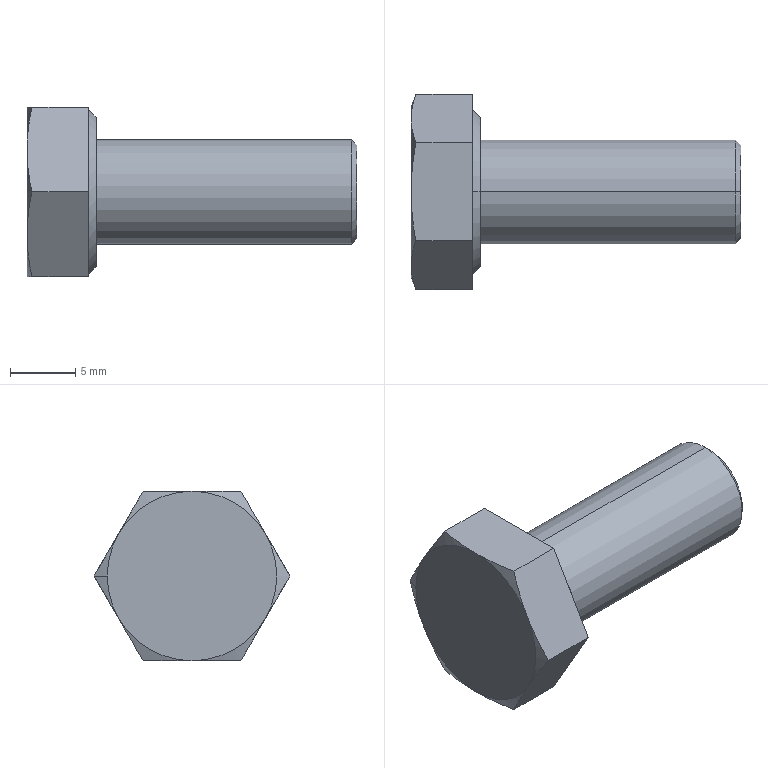Part | SolidWorks | features BaseBody 1, MoveFace 1 | 1 solid | 23 faces | box 25.3 x 15.011 x 13 mm | volume 1758 mm3 | cone 11 | plane 10 | cylinder 2 | commonest cylinder face diameters 8 x2
STEP:
#1=CARTESIAN_POINT('',(24.9,0.,4.));
#2=VERTEX_POINT('',#1);
#3=CARTESIAN_POINT('',(24.9,0.,-4.));
#4=VERTEX_POINT('',#3);
#5=CARTESIAN_POINT('',(24.9,0.,0.));
#6=DIRECTION('',(-1.,0.,0.));
#7=DIRECTION('',(0.,0.,1.));
#8=AXIS2_PLACEMENT_3D('',#5,#6,#7);
#9=CIRCLE('',#8,4.);
#10=EDGE_CURVE('',#2,#4,#9,.T.);
#11=ORIENTED_EDGE('',*,*,#10,.T.);
#12=CARTESIAN_POINT('',(5.3,0.,-4.));
#13=VERTEX_POINT('',#12);
#14=CARTESIAN_POINT('',(45.3,0.,-4.));
#15=DIRECTION('',(-1.,0.,0.));
#16=VECTOR('',#15,1000.);
#17=LINE('',#14,#16);
#18=EDGE_CURVE('',#4,#13,#17,.T.);
#19=ORIENTED_EDGE('',*,*,#18,.T.);
#20=CARTESIAN_POINT('',(5.3,0.,4.));
#21=VERTEX_POINT('',#20);
#22=CARTESIAN_POINT('',(5.3,0.,0.));
#23=DIRECTION('',(1.,0.,0.));
#24=DIRECTION('',(0.,0.,1.));
#25=AXIS2_PLACEMENT_3D('',#22,#23,#24);
#26=CIRCLE('',#25,4.);
#27=EDGE_CURVE('',#13,#21,#26,.T.);
#28=ORIENTED_EDGE('',*,*,#27,.T.);
#29=CARTESIAN_POINT('',(45.3,0.,4.));
#30=DIRECTION('',(-1.,0.,0.));
#31=VECTOR('',#30,1000.);
#32=LINE('',#29,#31);
#33=EDGE_CURVE('',#2,#21,#32,.T.);
#34=ORIENTED_EDGE('',*,*,#33,.F.);
#35=EDGE_LOOP('',(#11,#19,#28,#34));
#36=FACE_OUTER_BOUND('',#35,.T.);
#37=CARTESIAN_POINT('',(45.3,0.,0.));
#38=DIRECTION('',(-1.,0.,0.));
#39=DIRECTION('',(0.,0.,1.));
#40=AXIS2_PLACEMENT_3D('',#37,#38,#39);
#41=CYLINDRICAL_SURFACE('',#40,4.);
#42=ADVANCED_FACE('',(#36),#41,.T.);
#43=CARTESIAN_POINT('',(25.3,0.,3.6));
#44=VERTEX_POINT('',#43);
#45=CARTESIAN_POINT('',(25.3,0.,-3.6));
#46=VERTEX_POINT('',#45);
#47=CARTESIAN_POINT('',(25.3,0.,0.));
#48=DIRECTION('',(-1.,0.,0.));
#49=DIRECTION('',(0.,0.,1.));
#50=AXIS2_PLACEMENT_3D('',#47,#48,#49);
#51=CIRCLE('',#50,3.6);
#52=EDGE_CURVE('',#44,#46,#51,.T.);
#53=ORIENTED_EDGE('',*,*,#52,.T.);
#54=CARTESIAN_POINT('',(24.9,0.,-4.));
#55=DIRECTION('',(-0.7071,0.,-0.7071));
#56=VECTOR('',#55,1000.);
#57=LINE('',#54,#56);
#58=EDGE_CURVE('',#46,#4,#57,.T.);
#59=ORIENTED_EDGE('',*,*,#58,.T.);
#60=ORIENTED_EDGE('',*,*,#10,.F.);
#61=CARTESIAN_POINT('',(24.9,0.,4.));
#62=DIRECTION('',(-0.7071,0.,0.7071));
#63=VECTOR('',#62,1000.);
#64=LINE('',#61,#63);
#65=EDGE_CURVE('',#44,#2,#64,.T.);
#66=ORIENTED_EDGE('',*,*,#65,.F.);
#67=EDGE_LOOP('',(#53,#59,#60,#66));
#68=FACE_OUTER_BOUND('',#67,.T.);
#69=CARTESIAN_POINT('',(24.9,0.,0.));
#70=DIRECTION('',(-1.,0.,0.));
#71=DIRECTION('',(0.,0.,1.));
#72=AXIS2_PLACEMENT_3D('',#69,#70,#71);
#73=CONICAL_SURFACE('',#72,4.,0.7854);
#74=ADVANCED_FACE('',(#68),#73,.T.);
#75=CARTESIAN_POINT('',(5.3,0.,5.735));
#76=VERTEX_POINT('',#75);
#77=CARTESIAN_POINT('',(5.3,0.,-5.735));
#78=VERTEX_POINT('',#77);
#79=CARTESIAN_POINT('',(5.3,0.,0.));
#80=DIRECTION('',(-1.,0.,0.));
#81=DIRECTION('',(0.,0.,1.));
#82=AXIS2_PLACEMENT_3D('',#79,#80,#81);
#83=CIRCLE('',#82,5.735);
#84=EDGE_CURVE('',#76,#78,#83,.T.);
#85=ORIENTED_EDGE('',*,*,#84,.T.);
#86=CARTESIAN_POINT('',(4.7,0.,-6.335));
#87=VERTEX_POINT('',#86);
#88=CARTESIAN_POINT('',(4.7,0.,-6.335));
#89=DIRECTION('',(-0.7071,0.,-0.7071));
#90=VECTOR('',#89,1000.);
#91=LINE('',#88,#90);
#92=EDGE_CURVE('',#78,#87,#91,.T.);
#93=ORIENTED_EDGE('',*,*,#92,.T.);
#94=CARTESIAN_POINT('',(4.7,0.,6.335));
#95=VERTEX_POINT('',#94);
#96=CARTESIAN_POINT('',(4.7,0.,0.));
#97=DIRECTION('',(1.,0.,0.));
#98=DIRECTION('',(0.,0.,1.));
#99=AXIS2_PLACEMENT_3D('',#96,#97,#98);
#100=CIRCLE('',#99,6.335);
#101=EDGE_CURVE('',#87,#95,#100,.T.);
#102=ORIENTED_EDGE('',*,*,#101,.T.);
#103=CARTESIAN_POINT('',(4.7,0.,6.335));
#104=DIRECTION('',(-0.7071,0.,0.7071));
#105=VECTOR('',#104,1000.);
#106=LINE('',#103,#105);
#107=EDGE_CURVE('',#76,#95,#106,.T.);
#108=ORIENTED_EDGE('',*,*,#107,.F.);
#109=EDGE_LOOP('',(#85,#93,#102,#108));
#110=FACE_OUTER_BOUND('',#109,.T.);
#111=CARTESIAN_POINT('',(4.7,0.,0.));
#112=DIRECTION('',(-1.,0.,0.));
#113=DIRECTION('',(0.,0.,1.));
#114=AXIS2_PLACEMENT_3D('',#111,#112,#113);
#115=CONICAL_SURFACE('',#114,6.335,0.7854);
#116=ADVANCED_FACE('',(#110),#115,.T.);
#117=CARTESIAN_POINT('',(0.,5.629,-3.25));
#118=VERTEX_POINT('',#117);
#119=CARTESIAN_POINT('',(0.,6.5,0.));
#120=VERTEX_POINT('',#119);
#121=CARTESIAN_POINT('',(0.,0.,0.));
#122=DIRECTION('',(1.,0.,0.));
#123=DIRECTION('',(0.,1.,0.));
#124=AXIS2_PLACEMENT_3D('',#121,#122,#123);
#125=CIRCLE('',#124,6.5);
#126=EDGE_CURVE('',#118,#120,#125,.T.);
#127=ORIENTED_EDGE('',*,*,#126,.T.);
#128=CARTESIAN_POINT('',(0.366,7.506,0.));
#129=VERTEX_POINT('',#128);
#130=CARTESIAN_POINT('',(0.3682,7.512,0.));
#131=DIRECTION('',(0.342,0.9397,0.));
#132=VECTOR('',#131,1000.);
#133=LINE('',#130,#132);
#134=EDGE_CURVE('',#120,#129,#133,.T.);
#135=ORIENTED_EDGE('',*,*,#134,.T.);
#136=CARTESIAN_POINT('',(0.366,7.506,0.));
#137=CARTESIAN_POINT('',(0.1402,6.885,-1.075));
#138=CARTESIAN_POINT('',(0.,6.261,-2.156));
#139=CARTESIAN_POINT('',(0.,5.629,-3.25));
#140=B_SPLINE_CURVE_WITH_KNOTS('',3,(#136,#137,#138,#139),.UNSPECIFIED.,.F.,.F.,(4,4),(0.,0.003771),.UNSPECIFIED.);
#141=EDGE_CURVE('',#129,#118,#140,.T.);
#142=ORIENTED_EDGE('',*,*,#141,.T.);
#143=EDGE_LOOP('',(#127,#135,#142));
#144=FACE_OUTER_BOUND('',#143,.T.);
#145=CARTESIAN_POINT('',(0.3682,0.,0.));
#146=DIRECTION('',(1.,0.,0.));
#147=DIRECTION('',(0.,1.,0.));
#148=AXIS2_PLACEMENT_3D('',#145,#146,#147);
#149=CONICAL_SURFACE('',#148,7.512,1.222);
#150=ADVANCED_FACE('',(#144),#149,.T.);
#151=ORIENTED_EDGE('',*,*,#18,.F.);
#152=CARTESIAN_POINT('',(24.9,0.,0.));
#153=DIRECTION('',(-1.,0.,0.));
#154=DIRECTION('',(0.,0.,1.));
#155=AXIS2_PLACEMENT_3D('',#152,#153,#154);
#156=CIRCLE('',#155,4.);
#157=EDGE_CURVE('',#4,#2,#156,.T.);
#158=ORIENTED_EDGE('',*,*,#157,.T.);
#159=ORIENTED_EDGE('',*,*,#33,.T.);
#160=CARTESIAN_POINT('',(5.3,0.,0.));
#161=DIRECTION('',(1.,0.,0.));
#162=DIRECTION('',(0.,0.,1.));
#163=AXIS2_PLACEMENT_3D('',#160,#161,#162);
#164=CIRCLE('',#163,4.);
#165=EDGE_CURVE('',#21,#13,#164,.T.);
#166=ORIENTED_EDGE('',*,*,#165,.T.);
#167=EDGE_LOOP('',(#151,#158,#159,#166));
#168=FACE_OUTER_BOUND('',#167,.T.);
#169=CARTESIAN_POINT('',(45.3,0.,0.));
#170=DIRECTION('',(-1.,0.,0.));
#171=DIRECTION('',(0.,0.,1.));
#172=AXIS2_PLACEMENT_3D('',#169,#170,#171);
#173=CYLINDRICAL_SURFACE('',#172,4.);
#174=ADVANCED_FACE('',(#168),#173,.T.);
#175=ORIENTED_EDGE('',*,*,#165,.F.);
#176=ORIENTED_EDGE('',*,*,#27,.F.);
#177=EDGE_LOOP('',(#175,#176));
#178=FACE_BOUND('',#177,.T.);
#179=ORIENTED_EDGE('',*,*,#84,.F.);
#180=CARTESIAN_POINT('',(5.3,0.,0.));
#181=DIRECTION('',(-1.,0.,0.));
#182=DIRECTION('',(0.,0.,1.));
#183=AXIS2_PLACEMENT_3D('',#180,#181,#182);
#184=CIRCLE('',#183,5.735);
#185=EDGE_CURVE('',#78,#76,#184,.T.);
#186=ORIENTED_EDGE('',*,*,#185,.F.);
#187=EDGE_LOOP('',(#179,#186));
#188=FACE_OUTER_BOUND('',#187,.T.);
#189=CARTESIAN_POINT('',(5.3,0.,13.));
#190=DIRECTION('',(-1.,0.,0.));
#191=DIRECTION('',(0.,0.,1.));
#192=AXIS2_PLACEMENT_3D('',#189,#190,#191);
#193=PLANE('',#192);
#194=ADVANCED_FACE('',(#178,#188),#193,.F.);
#195=ORIENTED_EDGE('',*,*,#58,.F.);
#196=CARTESIAN_POINT('',(25.3,0.,0.));
#197=DIRECTION('',(-1.,0.,0.));
#198=DIRECTION('',(0.,0.,1.));
#199=AXIS2_PLACEMENT_3D('',#196,#197,#198);
#200=CIRCLE('',#199,3.6);
#201=EDGE_CURVE('',#46,#44,#200,.T.);
#202=ORIENTED_EDGE('',*,*,#201,.T.);
#203=ORIENTED_EDGE('',*,*,#65,.T.);
#204=ORIENTED_EDGE('',*,*,#157,.F.);
#205=EDGE_LOOP('',(#195,#202,#203,#204));
#206=FACE_OUTER_BOUND('',#205,.T.);
#207=CARTESIAN_POINT('',(24.9,0.,0.));
#208=DIRECTION('',(-1.,0.,0.));
#209=DIRECTION('',(0.,0.,1.));
#210=AXIS2_PLACEMENT_3D('',#207,#208,#209);
#211=CONICAL_SURFACE('',#210,4.,0.7854);
#212=ADVANCED_FACE('',(#206),#211,.T.);
#213=ORIENTED_EDGE('',*,*,#92,.F.);
#214=ORIENTED_EDGE('',*,*,#185,.T.);
#215=ORIENTED_EDGE('',*,*,#107,.T.);
#216=CARTESIAN_POINT('',(4.7,0.,0.));
#217=DIRECTION('',(1.,0.,0.));
#218=DIRECTION('',(0.,0.,1.));
#219=AXIS2_PLACEMENT_3D('',#216,#217,#218);
#220=CIRCLE('',#219,6.335);
#221=EDGE_CURVE('',#95,#87,#220,.T.);
#222=ORIENTED_EDGE('',*,*,#221,.T.);
#223=EDGE_LOOP('',(#213,#214,#215,#222));
#224=FACE_OUTER_BOUND('',#223,.T.);
#225=CARTESIAN_POINT('',(4.7,0.,0.));
#226=DIRECTION('',(-1.,0.,0.));
#227=DIRECTION('',(0.,0.,1.));
#228=AXIS2_PLACEMENT_3D('',#225,#226,#227);
#229=CONICAL_SURFACE('',#228,6.335,0.7854);
#230=ADVANCED_FACE('',(#224),#229,.T.);
#231=ORIENTED_EDGE('',*,*,#52,.F.);
#232=ORIENTED_EDGE('',*,*,#201,.F.);
#233=EDGE_LOOP('',(#231,#232));
#234=FACE_OUTER_BOUND('',#233,.T.);
#235=CARTESIAN_POINT('',(25.3,0.,0.));
#236=DIRECTION('',(1.,0.,0.));
#237=DIRECTION('',(0.,0.,-1.));
#238=AXIS2_PLACEMENT_3D('',#235,#236,#237);
#239=PLANE('',#238);
#240=ADVANCED_FACE('',(#234),#239,.T.);
#241=CARTESIAN_POINT('',(4.7,7.506,0.));
#242=VERTEX_POINT('',#241);
#243=CARTESIAN_POINT('',(4.7,3.753,6.5));
#244=VERTEX_POINT('',#243);
#245=CARTESIAN_POINT('',(4.7,7.506,0.));
#246=DIRECTION('',(0.,-0.5,0.866));
#247=VECTOR('',#246,1000.);
#248=LINE('',#245,#247);
#249=EDGE_CURVE('',#242,#244,#248,.T.);
#250=ORIENTED_EDGE('',*,*,#249,.T.);
#251=CARTESIAN_POINT('',(4.7,-3.753,6.5));
#252=VERTEX_POINT('',#251);
#253=CARTESIAN_POINT('',(4.7,6.335,6.5));
#254=DIRECTION('',(0.,-1.,0.));
#255=VECTOR('',#254,1000.);
#256=LINE('',#253,#255);
#257=EDGE_CURVE('',#244,#252,#256,.T.);
#258=ORIENTED_EDGE('',*,*,#257,.T.);
#259=CARTESIAN_POINT('',(4.7,-7.506,0.));
#260=VERTEX_POINT('',#259);
#261=CARTESIAN_POINT('',(4.7,-3.753,6.5));
#262=DIRECTION('',(0.,-0.5,-0.866));
#263=VECTOR('',#262,1000.);
#264=LINE('',#261,#263);
#265=EDGE_CURVE('',#252,#260,#264,.T.);
#266=ORIENTED_EDGE('',*,*,#265,.T.);
#267=CARTESIAN_POINT('',(4.7,-3.753,-6.5));
#268=VERTEX_POINT('',#267);
#269=CARTESIAN_POINT('',(4.7,-7.506,0.));
#270=DIRECTION('',(0.,0.5,-0.866));
#271=VECTOR('',#270,1000.);
#272=LINE('',#269,#271);
#273=EDGE_CURVE('',#260,#268,#272,.T.);
#274=ORIENTED_EDGE('',*,*,#273,.T.);
#275=CARTESIAN_POINT('',(4.7,3.753,-6.5));
#276=VERTEX_POINT('',#275);
#277=CARTESIAN_POINT('',(4.7,6.335,-6.5));
#278=DIRECTION('',(0.,1.,0.));
#279=VECTOR('',#278,1000.);
#280=LINE('',#277,#279);
#281=EDGE_CURVE('',#268,#276,#280,.T.);
#282=ORIENTED_EDGE('',*,*,#281,.T.);
#283=CARTESIAN_POINT('',(4.7,3.753,-6.5));
#284=DIRECTION('',(0.,0.5,0.866));
#285=VECTOR('',#284,1000.);
#286=LINE('',#283,#285);
#287=EDGE_CURVE('',#276,#242,#286,.T.);
#288=ORIENTED_EDGE('',*,*,#287,.T.);
#289=EDGE_LOOP('',(#250,#258,#266,#274,#282,#288));
#290=FACE_OUTER_BOUND('',#289,.T.);
#291=ORIENTED_EDGE('',*,*,#221,.F.);
#292=ORIENTED_EDGE('',*,*,#101,.F.);
#293=EDGE_LOOP('',(#291,#292));
#294=FACE_BOUND('',#293,.T.);
#295=CARTESIAN_POINT('',(4.7,6.335,0.));
#296=DIRECTION('',(1.,0.,0.));
#297=DIRECTION('',(0.,0.,-1.));
#298=AXIS2_PLACEMENT_3D('',#295,#296,#297);
#299=PLANE('',#298);
#300=ADVANCED_FACE('',(#290,#294),#299,.T.);
#301=CARTESIAN_POINT('',(0.366,-3.753,6.5));
#302=VERTEX_POINT('',#301);
#303=CARTESIAN_POINT('',(5.3,-3.753,6.5));
#304=DIRECTION('',(-1.,0.,0.));
#305=VECTOR('',#304,1000.);
#306=LINE('',#303,#305);
#307=EDGE_CURVE('',#252,#302,#306,.T.);
#308=ORIENTED_EDGE('',*,*,#307,.F.);
#309=ORIENTED_EDGE('',*,*,#257,.F.);
#310=CARTESIAN_POINT('',(0.366,3.753,6.5));
#311=VERTEX_POINT('',#310);
#312=CARTESIAN_POINT('',(5.3,3.753,6.5));
#313=DIRECTION('',(1.,0.,0.));
#314=VECTOR('',#313,1000.);
#315=LINE('',#312,#314);
#316=EDGE_CURVE('',#311,#244,#315,.T.);
#317=ORIENTED_EDGE('',*,*,#316,.F.);
#318=CARTESIAN_POINT('',(0.,0.,6.5));
#319=VERTEX_POINT('',#318);
#320=CARTESIAN_POINT('',(0.,0.,6.5));
#321=CARTESIAN_POINT('',(0.,1.263,6.5));
#322=CARTESIAN_POINT('',(0.1402,2.512,6.5));
#323=CARTESIAN_POINT('',(0.366,3.753,6.5));
#324=B_SPLINE_CURVE_WITH_KNOTS('',3,(#320,#321,#322,#323),.UNSPECIFIED.,.F.,.F.,(4,4),(0.,0.003771),.UNSPECIFIED.);
#325=EDGE_CURVE('',#319,#311,#324,.T.);
#326=ORIENTED_EDGE('',*,*,#325,.F.);
#327=CARTESIAN_POINT('',(0.366,-3.753,6.5));
#328=CARTESIAN_POINT('',(0.1402,-2.512,6.5));
#329=CARTESIAN_POINT('',(0.,-1.263,6.5));
#330=CARTESIAN_POINT('',(0.,0.,6.5));
#331=B_SPLINE_CURVE_WITH_KNOTS('',3,(#327,#328,#329,#330),.UNSPECIFIED.,.F.,.F.,(4,4),(0.,0.003771),.UNSPECIFIED.);
#332=EDGE_CURVE('',#302,#319,#331,.T.);
#333=ORIENTED_EDGE('',*,*,#332,.F.);
#334=EDGE_LOOP('',(#308,#309,#317,#326,#333));
#335=FACE_OUTER_BOUND('',#334,.T.);
#336=CARTESIAN_POINT('',(5.3,3.753,6.5));
#337=DIRECTION('',(0.,0.,-1.));
#338=DIRECTION('',(-1.,0.,0.));
#339=AXIS2_PLACEMENT_3D('',#336,#337,#338);
#340=PLANE('',#339);
#341=ADVANCED_FACE('',(#335),#340,.F.);
#342=ORIENTED_EDGE('',*,*,#316,.T.);
#343=ORIENTED_EDGE('',*,*,#249,.F.);
#344=CARTESIAN_POINT('',(5.3,7.506,0.));
#345=DIRECTION('',(1.,0.,0.));
#346=VECTOR('',#345,1000.);
#347=LINE('',#344,#346);
#348=EDGE_CURVE('',#129,#242,#347,.T.);
#349=ORIENTED_EDGE('',*,*,#348,.F.);
#350=CARTESIAN_POINT('',(0.,5.629,3.25));
#351=VERTEX_POINT('',#350);
#352=CARTESIAN_POINT('',(0.,5.629,3.25));
#353=CARTESIAN_POINT('',(0.,6.261,2.156));
#354=CARTESIAN_POINT('',(0.1402,6.885,1.075));
#355=CARTESIAN_POINT('',(0.366,7.506,0.));
#356=B_SPLINE_CURVE_WITH_KNOTS('',3,(#352,#353,#354,#355),.UNSPECIFIED.,.F.,.F.,(4,4),(0.,0.003771),.UNSPECIFIED.);
#357=EDGE_CURVE('',#351,#129,#356,.T.);
#358=ORIENTED_EDGE('',*,*,#357,.F.);
#359=CARTESIAN_POINT('',(0.366,3.753,6.5));
#360=CARTESIAN_POINT('',(0.1402,4.373,5.425));
#361=CARTESIAN_POINT('',(0.,4.998,4.344));
#362=CARTESIAN_POINT('',(0.,5.629,3.25));
#363=B_SPLINE_CURVE_WITH_KNOTS('',3,(#359,#360,#361,#362),.UNSPECIFIED.,.F.,.F.,(4,4),(0.,0.003771),.UNSPECIFIED.);
#364=EDGE_CURVE('',#311,#351,#363,.T.);
#365=ORIENTED_EDGE('',*,*,#364,.F.);
#366=EDGE_LOOP('',(#342,#343,#349,#358,#365));
#367=FACE_OUTER_BOUND('',#366,.T.);
#368=CARTESIAN_POINT('',(5.3,7.506,0.));
#369=DIRECTION('',(0.,-0.866,-0.5));
#370=DIRECTION('',(0.,0.5,-0.866));
#371=AXIS2_PLACEMENT_3D('',#368,#369,#370);
#372=PLANE('',#371);
#373=ADVANCED_FACE('',(#367),#372,.F.);
#374=ORIENTED_EDGE('',*,*,#348,.T.);
#375=ORIENTED_EDGE('',*,*,#287,.F.);
#376=CARTESIAN_POINT('',(0.366,3.753,-6.5));
#377=VERTEX_POINT('',#376);
#378=CARTESIAN_POINT('',(5.3,3.753,-6.5));
#379=DIRECTION('',(1.,0.,0.));
#380=VECTOR('',#379,1000.);
#381=LINE('',#378,#380);
#382=EDGE_CURVE('',#377,#276,#381,.T.);
#383=ORIENTED_EDGE('',*,*,#382,.F.);
#384=CARTESIAN_POINT('',(0.,5.629,-3.25));
#385=CARTESIAN_POINT('',(0.,4.998,-4.344));
#386=CARTESIAN_POINT('',(0.1402,4.373,-5.425));
#387=CARTESIAN_POINT('',(0.366,3.753,-6.5));
#388=B_SPLINE_CURVE_WITH_KNOTS('',3,(#384,#385,#386,#387),.UNSPECIFIED.,.F.,.F.,(4,4),(0.,0.003771),.UNSPECIFIED.);
#389=EDGE_CURVE('',#118,#377,#388,.T.);
#390=ORIENTED_EDGE('',*,*,#389,.F.);
#391=ORIENTED_EDGE('',*,*,#141,.F.);
#392=EDGE_LOOP('',(#374,#375,#383,#390,#391));
#393=FACE_OUTER_BOUND('',#392,.T.);
#394=CARTESIAN_POINT('',(5.3,3.753,-6.5));
#395=DIRECTION('',(0.,-0.866,0.5));
#396=DIRECTION('',(0.,-0.5,-0.866));
#397=AXIS2_PLACEMENT_3D('',#394,#395,#396);
#398=PLANE('',#397);
#399=ADVANCED_FACE('',(#393),#398,.F.);
#400=ORIENTED_EDGE('',*,*,#382,.T.);
#401=ORIENTED_EDGE('',*,*,#281,.F.);
#402=CARTESIAN_POINT('',(0.366,-3.753,-6.5));
#403=VERTEX_POINT('',#402);
#404=CARTESIAN_POINT('',(5.3,-3.753,-6.5));
#405=DIRECTION('',(1.,0.,0.));
#406=VECTOR('',#405,1000.);
#407=LINE('',#404,#406);
#408=EDGE_CURVE('',#403,#268,#407,.T.);
#409=ORIENTED_EDGE('',*,*,#408,.F.);
#410=CARTESIAN_POINT('',(0.,0.,-6.5));
#411=VERTEX_POINT('',#410);
#412=CARTESIAN_POINT('',(0.,0.,-6.5));
#413=CARTESIAN_POINT('',(0.,-1.263,-6.5));
#414=CARTESIAN_POINT('',(0.1402,-2.512,-6.5));
#415=CARTESIAN_POINT('',(0.366,-3.753,-6.5));
#416=B_SPLINE_CURVE_WITH_KNOTS('',3,(#412,#413,#414,#415),.UNSPECIFIED.,.F.,.F.,(4,4),(0.,0.003771),.UNSPECIFIED.);
#417=EDGE_CURVE('',#411,#403,#416,.T.);
#418=ORIENTED_EDGE('',*,*,#417,.F.);
#419=CARTESIAN_POINT('',(0.366,3.753,-6.5));
#420=CARTESIAN_POINT('',(0.1402,2.512,-6.5));
#421=CARTESIAN_POINT('',(0.,1.263,-6.5));
#422=CARTESIAN_POINT('',(0.,0.,-6.5));
#423=B_SPLINE_CURVE_WITH_KNOTS('',3,(#419,#420,#421,#422),.UNSPECIFIED.,.F.,.F.,(4,4),(0.,0.003771),.UNSPECIFIED.);
#424=EDGE_CURVE('',#377,#411,#423,.T.);
#425=ORIENTED_EDGE('',*,*,#424,.F.);
#426=EDGE_LOOP('',(#400,#401,#409,#418,#425));
#427=FACE_OUTER_BOUND('',#426,.T.);
#428=CARTESIAN_POINT('',(5.3,-3.753,-6.5));
#429=DIRECTION('',(0.,0.,1.));
#430=DIRECTION('',(1.,0.,0.));
#431=AXIS2_PLACEMENT_3D('',#428,#429,#430);
#432=PLANE('',#431);
#433=ADVANCED_FACE('',(#427),#432,.F.);
#434=ORIENTED_EDGE('',*,*,#408,.T.);
#435=ORIENTED_EDGE('',*,*,#273,.F.);
#436=CARTESIAN_POINT('',(0.366,-7.506,0.));
#437=VERTEX_POINT('',#436);
#438=CARTESIAN_POINT('',(5.3,-7.506,0.));
#439=DIRECTION('',(1.,0.,0.));
#440=VECTOR('',#439,1000.);
#441=LINE('',#438,#440);
#442=EDGE_CURVE('',#437,#260,#441,.T.);
#443=ORIENTED_EDGE('',*,*,#442,.F.);
#444=CARTESIAN_POINT('',(0.,-5.629,-3.25));
#445=VERTEX_POINT('',#444);
#446=CARTESIAN_POINT('',(0.,-5.629,-3.25));
#447=CARTESIAN_POINT('',(0.,-6.261,-2.156));
#448=CARTESIAN_POINT('',(0.1402,-6.885,-1.075));
#449=CARTESIAN_POINT('',(0.366,-7.506,0.));
#450=B_SPLINE_CURVE_WITH_KNOTS('',3,(#446,#447,#448,#449),.UNSPECIFIED.,.F.,.F.,(4,4),(0.,0.003771),.UNSPECIFIED.);
#451=EDGE_CURVE('',#445,#437,#450,.T.);
#452=ORIENTED_EDGE('',*,*,#451,.F.);
#453=CARTESIAN_POINT('',(0.366,-3.753,-6.5));
#454=CARTESIAN_POINT('',(0.1402,-4.373,-5.425));
#455=CARTESIAN_POINT('',(0.,-4.998,-4.344));
#456=CARTESIAN_POINT('',(0.,-5.629,-3.25));
#457=B_SPLINE_CURVE_WITH_KNOTS('',3,(#453,#454,#455,#456),.UNSPECIFIED.,.F.,.F.,(4,4),(0.,0.003771),.UNSPECIFIED.);
#458=EDGE_CURVE('',#403,#445,#457,.T.);
#459=ORIENTED_EDGE('',*,*,#458,.F.);
#460=EDGE_LOOP('',(#434,#435,#443,#452,#459));
#461=FACE_OUTER_BOUND('',#460,.T.);
#462=CARTESIAN_POINT('',(5.3,-7.506,0.));
#463=DIRECTION('',(0.,0.866,0.5));
#464=DIRECTION('',(0.,-0.5,0.866));
#465=AXIS2_PLACEMENT_3D('',#462,#463,#464);
#466=PLANE('',#465);
#467=ADVANCED_FACE('',(#461),#466,.F.);
#468=ORIENTED_EDGE('',*,*,#442,.T.);
#469=ORIENTED_EDGE('',*,*,#265,.F.);
#470=ORIENTED_EDGE('',*,*,#307,.T.);
#471=CARTESIAN_POINT('',(0.,-5.629,3.25));
#472=VERTEX_POINT('',#471);
#473=CARTESIAN_POINT('',(0.,-5.629,3.25));
#474=CARTESIAN_POINT('',(0.,-4.998,4.344));
#475=CARTESIAN_POINT('',(0.1402,-4.373,5.425));
#476=CARTESIAN_POINT('',(0.366,-3.753,6.5));
#477=B_SPLINE_CURVE_WITH_KNOTS('',3,(#473,#474,#475,#476),.UNSPECIFIED.,.F.,.F.,(4,4),(0.,0.003771),.UNSPECIFIED.);
#478=EDGE_CURVE('',#472,#302,#477,.T.);
#479=ORIENTED_EDGE('',*,*,#478,.F.);
#480=CARTESIAN_POINT('',(0.366,-7.506,0.));
#481=CARTESIAN_POINT('',(0.1402,-6.885,1.075));
#482=CARTESIAN_POINT('',(0.,-6.261,2.156));
#483=CARTESIAN_POINT('',(0.,-5.629,3.25));
#484=B_SPLINE_CURVE_WITH_KNOTS('',3,(#480,#481,#482,#483),.UNSPECIFIED.,.F.,.F.,(4,4),(0.,0.003771),.UNSPECIFIED.);
#485=EDGE_CURVE('',#437,#472,#484,.T.);
#486=ORIENTED_EDGE('',*,*,#485,.F.);
#487=EDGE_LOOP('',(#468,#469,#470,#479,#486));
#488=FACE_OUTER_BOUND('',#487,.T.);
#489=CARTESIAN_POINT('',(5.3,-3.753,6.5));
#490=DIRECTION('',(0.,0.866,-0.5));
#491=DIRECTION('',(0.,0.5,0.866));
#492=AXIS2_PLACEMENT_3D('',#489,#490,#491);
#493=PLANE('',#492);
#494=ADVANCED_FACE('',(#488),#493,.F.);
#495=ORIENTED_EDGE('',*,*,#332,.T.);
#496=CARTESIAN_POINT('',(0.,0.,0.));
#497=DIRECTION('',(1.,0.,0.));
#498=DIRECTION('',(0.,1.,0.));
#499=AXIS2_PLACEMENT_3D('',#496,#497,#498);
#500=CIRCLE('',#499,6.5);
#501=EDGE_CURVE('',#319,#472,#500,.T.);
#502=ORIENTED_EDGE('',*,*,#501,.T.);
#503=ORIENTED_EDGE('',*,*,#478,.T.);
#504=EDGE_LOOP('',(#495,#502,#503));
#505=FACE_OUTER_BOUND('',#504,.T.);
#506=CARTESIAN_POINT('',(0.3682,0.,0.));
#507=DIRECTION('',(1.,0.,0.));
#508=DIRECTION('',(0.,1.,0.));
#509=AXIS2_PLACEMENT_3D('',#506,#507,#508);
#510=CONICAL_SURFACE('',#509,7.512,1.222);
#511=ADVANCED_FACE('',(#505),#510,.T.);
#512=CARTESIAN_POINT('',(0.,0.,0.));
#513=DIRECTION('',(1.,0.,0.));
#514=DIRECTION('',(0.,1.,0.));
#515=AXIS2_PLACEMENT_3D('',#512,#513,#514);
#516=CIRCLE('',#515,6.5);
#517=EDGE_CURVE('',#351,#319,#516,.T.);
#518=ORIENTED_EDGE('',*,*,#517,.T.);
#519=ORIENTED_EDGE('',*,*,#325,.T.);
#520=ORIENTED_EDGE('',*,*,#364,.T.);
#521=EDGE_LOOP('',(#518,#519,#520));
#522=FACE_OUTER_BOUND('',#521,.T.);
#523=CARTESIAN_POINT('',(0.3682,0.,0.));
#524=DIRECTION('',(1.,0.,0.));
#525=DIRECTION('',(0.,1.,0.));
#526=AXIS2_PLACEMENT_3D('',#523,#524,#525);
#527=CONICAL_SURFACE('',#526,7.512,1.222);
#528=ADVANCED_FACE('',(#522),#527,.T.);
#529=ORIENTED_EDGE('',*,*,#134,.F.);
#530=CARTESIAN_POINT('',(0.,0.,0.));
#531=DIRECTION('',(1.,0.,0.));
#532=DIRECTION('',(0.,1.,0.));
#533=AXIS2_PLACEMENT_3D('',#530,#531,#532);
#534=CIRCLE('',#533,6.5);
#535=EDGE_CURVE('',#120,#351,#534,.T.);
#536=ORIENTED_EDGE('',*,*,#535,.T.);
#537=ORIENTED_EDGE('',*,*,#357,.T.);
#538=EDGE_LOOP('',(#529,#536,#537));
#539=FACE_OUTER_BOUND('',#538,.T.);
#540=CARTESIAN_POINT('',(0.3682,0.,0.));
#541=DIRECTION('',(1.,0.,0.));
#542=DIRECTION('',(0.,1.,0.));
#543=AXIS2_PLACEMENT_3D('',#540,#541,#542);
#544=CONICAL_SURFACE('',#543,7.512,1.222);
#545=ADVANCED_FACE('',(#539),#544,.T.);
#546=CARTESIAN_POINT('',(0.,0.,0.));
#547=DIRECTION('',(1.,0.,0.));
#548=DIRECTION('',(0.,1.,0.));
#549=AXIS2_PLACEMENT_3D('',#546,#547,#548);
#550=CIRCLE('',#549,6.5);
#551=EDGE_CURVE('',#411,#118,#550,.T.);
#552=ORIENTED_EDGE('',*,*,#551,.T.);
#553=ORIENTED_EDGE('',*,*,#389,.T.);
#554=ORIENTED_EDGE('',*,*,#424,.T.);
#555=EDGE_LOOP('',(#552,#553,#554));
#556=FACE_OUTER_BOUND('',#555,.T.);
#557=CARTESIAN_POINT('',(0.3682,0.,0.));
#558=DIRECTION('',(1.,0.,0.));
#559=DIRECTION('',(0.,1.,0.));
#560=AXIS2_PLACEMENT_3D('',#557,#558,#559);
#561=CONICAL_SURFACE('',#560,7.512,1.222);
#562=ADVANCED_FACE('',(#556),#561,.T.);
#563=ORIENTED_EDGE('',*,*,#458,.T.);
#564=CARTESIAN_POINT('',(0.,0.,0.));
#565=DIRECTION('',(1.,0.,0.));
#566=DIRECTION('',(0.,1.,0.));
#567=AXIS2_PLACEMENT_3D('',#564,#565,#566);
#568=CIRCLE('',#567,6.5);
#569=EDGE_CURVE('',#445,#411,#568,.T.);
#570=ORIENTED_EDGE('',*,*,#569,.T.);
#571=ORIENTED_EDGE('',*,*,#417,.T.);
#572=EDGE_LOOP('',(#563,#570,#571));
#573=FACE_OUTER_BOUND('',#572,.T.);
#574=CARTESIAN_POINT('',(0.3682,0.,0.));
#575=DIRECTION('',(1.,0.,0.));
#576=DIRECTION('',(0.,1.,0.));
#577=AXIS2_PLACEMENT_3D('',#574,#575,#576);
#578=CONICAL_SURFACE('',#577,7.512,1.222);
#579=ADVANCED_FACE('',(#573),#578,.T.);
#580=ORIENTED_EDGE('',*,*,#485,.T.);
#581=CARTESIAN_POINT('',(0.,0.,0.));
#582=DIRECTION('',(1.,0.,0.));
#583=DIRECTION('',(0.,1.,0.));
#584=AXIS2_PLACEMENT_3D('',#581,#582,#583);
#585=CIRCLE('',#584,6.5);
#586=EDGE_CURVE('',#472,#445,#585,.T.);
#587=ORIENTED_EDGE('',*,*,#586,.T.);
#588=ORIENTED_EDGE('',*,*,#451,.T.);
#589=EDGE_LOOP('',(#580,#587,#588));
#590=FACE_OUTER_BOUND('',#589,.T.);
#591=CARTESIAN_POINT('',(0.3682,0.,0.));
#592=DIRECTION('',(1.,0.,0.));
#593=DIRECTION('',(0.,1.,0.));
#594=AXIS2_PLACEMENT_3D('',#591,#592,#593);
#595=CONICAL_SURFACE('',#594,7.512,1.222);
#596=ADVANCED_FACE('',(#590),#595,.T.);
#597=ORIENTED_EDGE('',*,*,#569,.F.);
#598=ORIENTED_EDGE('',*,*,#586,.F.);
#599=ORIENTED_EDGE('',*,*,#501,.F.);
#600=ORIENTED_EDGE('',*,*,#517,.F.);
#601=ORIENTED_EDGE('',*,*,#535,.F.);
#602=ORIENTED_EDGE('',*,*,#126,.F.);
#603=ORIENTED_EDGE('',*,*,#551,.F.);
#604=EDGE_LOOP('',(#597,#598,#599,#600,#601,#602,#603));
#605=FACE_OUTER_BOUND('',#604,.T.);
#606=CARTESIAN_POINT('',(0.,0.,13.));
#607=DIRECTION('',(-1.,0.,0.));
#608=DIRECTION('',(0.,0.,1.));
#609=AXIS2_PLACEMENT_3D('',#606,#607,#608);
#610=PLANE('',#609);
#611=ADVANCED_FACE('',(#605),#610,.T.);
#612=CLOSED_SHELL('',(#42,#74,#116,#150,#174,#194,#212,#230,#240,#300,#341,#373,#399,#433,#467,#494,#511,#528,#545,#562,#579,#596,#611));
#613=MANIFOLD_SOLID_BREP('',#612);
#614=CARTESIAN_POINT('',(0.,0.,0.));
#615=DIRECTION('',(0.,0.,1.));
#616=DIRECTION('',(1.,0.,0.));
#617=AXIS2_PLACEMENT_3D('',#614,#615,#616);
#618=(LENGTH_UNIT()NAMED_UNIT(*)SI_UNIT(.MILLI.,.METRE.));
#619=UNCERTAINTY_MEASURE_WITH_UNIT(LENGTH_MEASURE(0.00001),#618,'','');
#620=(NAMED_UNIT(*)PLANE_ANGLE_UNIT()SI_UNIT($,.RADIAN.));
#621=(NAMED_UNIT(*)SI_UNIT($,.STERADIAN.)SOLID_ANGLE_UNIT());
#622=(GEOMETRIC_REPRESENTATION_CONTEXT(3)GLOBAL_UNCERTAINTY_ASSIGNED_CONTEXT((#619))GLOBAL_UNIT_ASSIGNED_CONTEXT((#618,#620,#621))REPRESENTATION_CONTEXT('',''));
#623=ADVANCED_BREP_SHAPE_REPRESENTATION('',(#613,#617),#622);